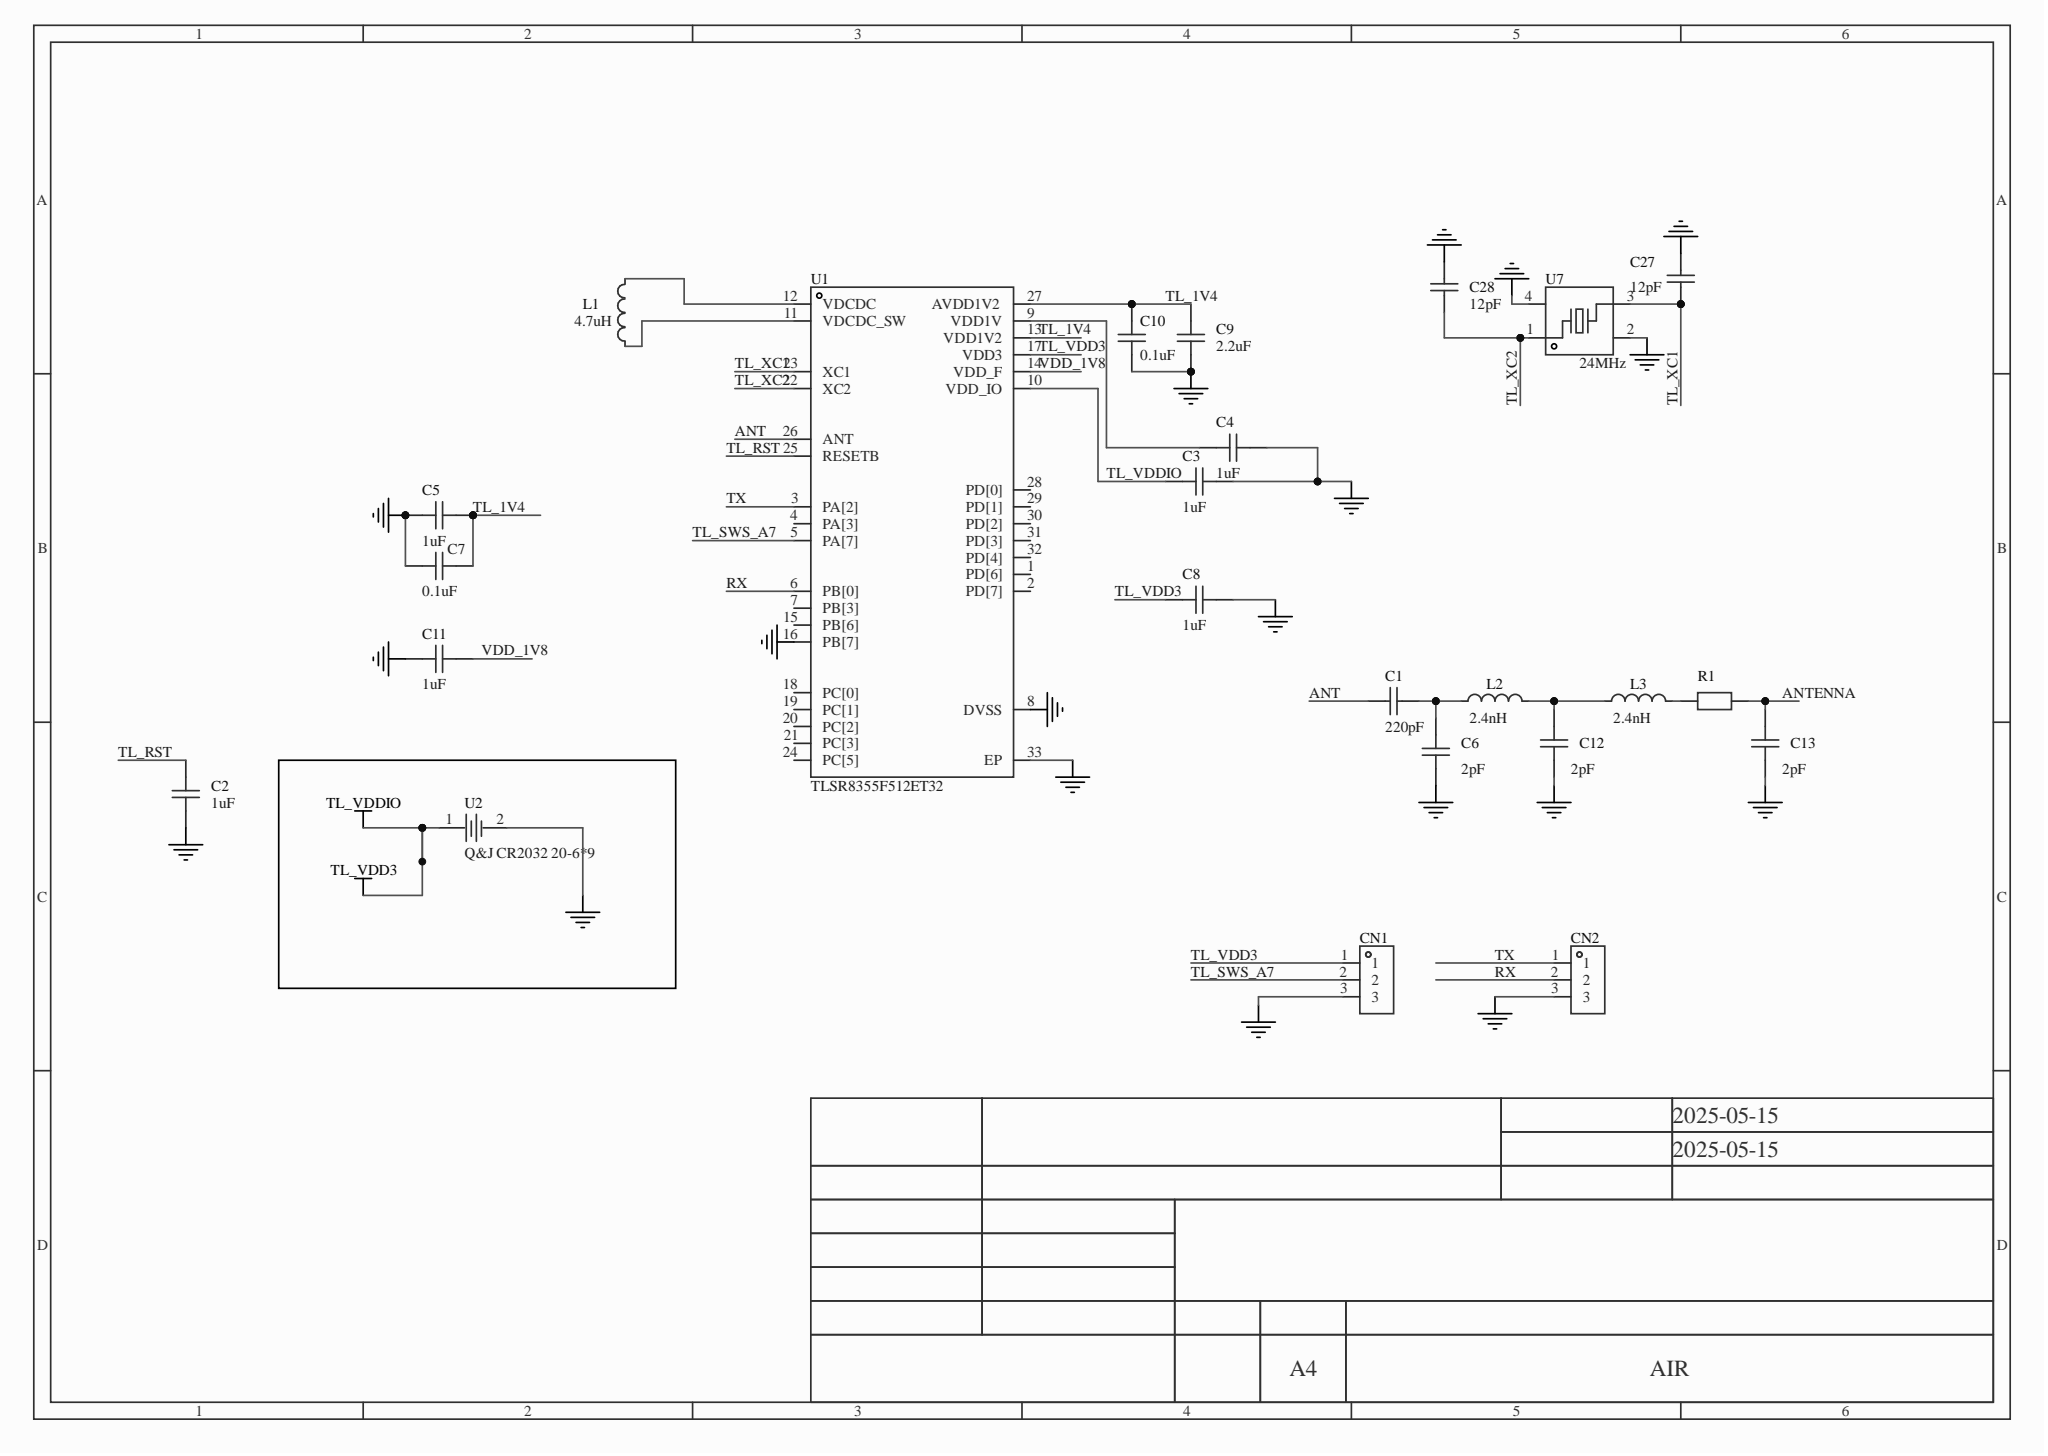Circuit board | Altium Designer | 24 parts | 18 nets
Bill of materials:
Comment,Description,Designator,Footprint,LibRef,Quantity
"220pF","","C1","C0402","CC0402KRX7R9BB221","1"
"1uF","","C2, C3, C4, C5, C8, C11","C0402","CL05A105KA5NQNC","6"
"2pF","","C6, C12, C13","C0402","CC0402CRNPO9BN2R0","3"
"0.1uF","","C7","C0603","CAP_0603","1"
"2.2uF","","C9","C0402","CL05A105KA5NQNC","1"
"0.1uF","","C10","C0402","CL05A105KA5NQNC","1"
"12pF","","C27, C28","C0402","0402CG120J500NT","2"
"","","CN1, CN2","HDR-TH_3P-P1.27-V-M-A","3Pin_1.27___","2"
"4.7uH","","L1","IND-SMD_L1.8-W1.2","SLC1608F4R7KTT","1"
"2.4nH","","L2, L3","L0402","LQG15HH2N4S02D","2"
"","","R1","R0402","SCR0402J0R","1"
"TLSR8355F512ET32","","U1","TQFN-32_L5.0-W5.0-P0.50-BL-EP3.5","TLSR8355F512ET32","1"
"Q&J CR2032 20-6*9","","U2","BAT-TH_CR2032","Q&J CR2032 20-6*9","1"
"24MHz","","U7","JWT1238","JWT1238","1"
Netlist (Protel format):
[
C1
C0402
220pF



]
[
C2
C0402
1uF



]
[
C3
C0402
1uF



]
[
C4
C0402
1uF



]
[
C5
C0402
1uF



]
[
C6
C0402
2pF



]
[
C7
C0603
0.1uF



]
[
C8
C0402
1uF



]
[
C9
C0402
2.2uF



]
[
C10
C0402
0.1uF



]
[
C11
C0402
1uF



]
[
C12
C0402
2pF



]
[
C13
C0402
2pF



]
[
C27
C0402
12pF



]
[
C28
C0402
12pF



]
[
CN1
HDR-TH_3P-P1.27-V-M-A




]
[
CN2
HDR-TH_3P-P1.27-V-M-A




]
[
L1
IND-SMD_L1.8-W1.2
4.7uH



]
[
L2
L0402
2.4nH



]
[
L3
L0402
2.4nH



]
[
R1
R0402




]
[
U1
TQFN-32_L5.0-W5.0-P0.50-BL-EP3.5
TLSR8355F512ET32



]
[
U2
BAT-TH_CR2032
Q&J CR2032 20-6*9



]
[
U7
JWT1238
24MHz



]
(
VDD_1V8
C11-2
U1-14
)
(
TX
CN2-1
U1-3
)
(
TL_XC2
C28-1
U1-22
U7-1
)
(
TL_XC1
C27-1
U1-23
U7-3
)
(
TL_VDD3
C3-2
C8-1
CN1-1
U1-10
U1-17
U2-1
)
(
TL_SWS_A7
CN1-2
U1-5
)
(
TL_RST
C2-2
U1-25
)
(
TL_1V4
C5-2
C7-2
C9-2
C10-2
U1-13
U1-27
)
(
RX
CN2-2
U1-6
)
(
NetL3_2
L3-2
R1-1
)
(
NetL1_2
L1-2
U1-12
)
(
NetL1_1
L1-1
U1-11
)
(
NetC12_2
C12-2
L2-2
L3-1
)
(
NetC4_2
C4-2
U1-9
)
(
NetC1_2
C1-2
C6-2
L2-1
)
(
GND
C2-1
C3-1
C4-1
C5-1
C6-1
C7-1
C8-2
C9-1
C10-1
C11-1
C12-1
C13-1
C27-2
C28-2
CN1-3
CN2-3
U1-8
U1-16
U1-33
U2-2
U7-2
U7-4
)
(
ANTENNA
C13-2
R1-2
)
(
ANT
C1-1
U1-26
)